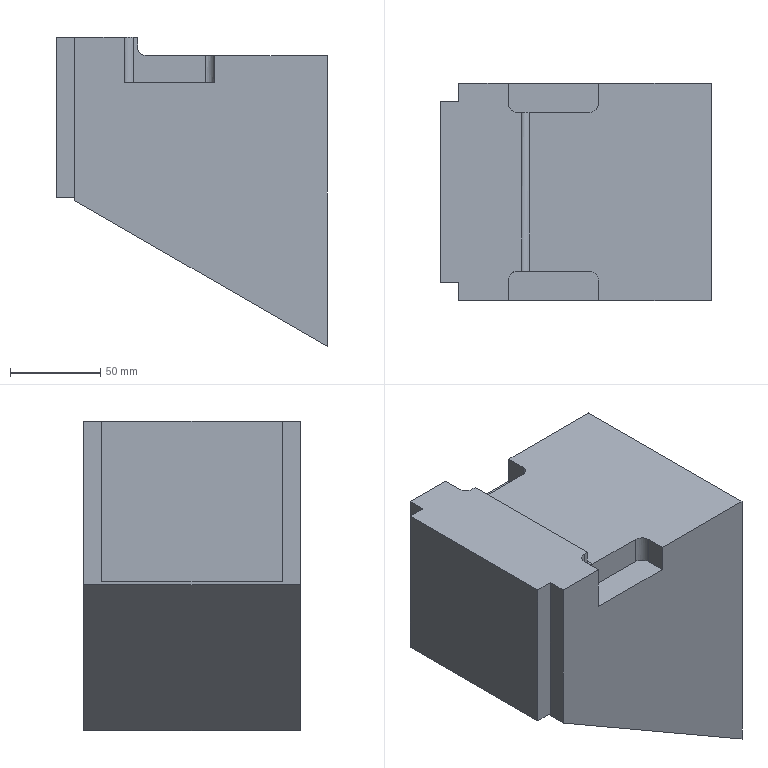Part | NX | features solid 2 | 1 solid | 25 faces | box 150 x 120 x 171.127 mm | volume 2133147 mm3 | plane 20 | cylinder 5 | commonest cylinder face diameters 10 x4 8 x1
STEP:
#1=CARTESIAN_POINT('',(-940.5,68.,-30.));
#2=VERTEX_POINT('',#1);
#3=CARTESIAN_POINT('',(-940.5,68.,-55.));
#4=VERTEX_POINT('',#3);
#5=CARTESIAN_POINT('',(-940.5,68.,-30.));
#6=CARTESIAN_POINT('',(-940.5,68.,-38.333));
#7=CARTESIAN_POINT('',(-940.5,68.,-46.667));
#8=CARTESIAN_POINT('',(-940.5,68.,-55.));
#9=B_SPLINE_CURVE_WITH_KNOTS('',3,(#5,#6,#7,#8),.UNSPECIFIED.,.F.,.F.,(4,4),(0.,1.),.UNSPECIFIED.);
#10=EDGE_CURVE('',#2,#4,#9,.T.);
#11=ORIENTED_EDGE('',*,*,#10,.T.);
#12=CARTESIAN_POINT('',(-890.5,68.,-55.));
#13=VERTEX_POINT('',#12);
#14=CARTESIAN_POINT('',(-940.5,68.,-55.));
#15=CARTESIAN_POINT('',(-923.833,68.,-55.));
#16=CARTESIAN_POINT('',(-907.167,68.,-55.));
#17=CARTESIAN_POINT('',(-890.5,68.,-55.));
#18=B_SPLINE_CURVE_WITH_KNOTS('',3,(#14,#15,#16,#17),.UNSPECIFIED.,.F.,.F.,(4,4),(0.,1.),.UNSPECIFIED.);
#19=EDGE_CURVE('',#4,#13,#18,.T.);
#20=ORIENTED_EDGE('',*,*,#19,.T.);
#21=CARTESIAN_POINT('',(-890.5,68.,-40.));
#22=VERTEX_POINT('',#21);
#23=CARTESIAN_POINT('',(-890.5,68.,-55.));
#24=CARTESIAN_POINT('',(-890.5,68.,-50.));
#25=CARTESIAN_POINT('',(-890.5,68.,-45.));
#26=CARTESIAN_POINT('',(-890.5,68.,-40.));
#27=B_SPLINE_CURVE_WITH_KNOTS('',3,(#23,#24,#25,#26),.UNSPECIFIED.,.F.,.F.,(4,4),(0.,1.),.UNSPECIFIED.);
#28=EDGE_CURVE('',#13,#22,#27,.T.);
#29=ORIENTED_EDGE('',*,*,#28,.T.);
#30=CARTESIAN_POINT('',(-828.,68.,-40.));
#31=VERTEX_POINT('',#30);
#32=CARTESIAN_POINT('',(-890.5,68.,-40.));
#33=CARTESIAN_POINT('',(-869.667,68.,-40.));
#34=CARTESIAN_POINT('',(-848.833,68.,-40.));
#35=CARTESIAN_POINT('',(-828.,68.,-40.));
#36=B_SPLINE_CURVE_WITH_KNOTS('',3,(#32,#33,#34,#35),.UNSPECIFIED.,.F.,.F.,(4,4),(0.,1.),.UNSPECIFIED.);
#37=EDGE_CURVE('',#22,#31,#36,.T.);
#38=ORIENTED_EDGE('',*,*,#37,.T.);
#39=CARTESIAN_POINT('',(-828.,68.,-201.127));
#40=VERTEX_POINT('',#39);
#41=CARTESIAN_POINT('',(-828.,68.,-40.));
#42=CARTESIAN_POINT('',(-828.,68.,-93.709));
#43=CARTESIAN_POINT('',(-828.,68.,-147.418));
#44=CARTESIAN_POINT('',(-828.,68.,-201.127));
#45=B_SPLINE_CURVE_WITH_KNOTS('',3,(#41,#42,#43,#44),.UNSPECIFIED.,.F.,.F.,(4,4),(0.,1.),.UNSPECIFIED.);
#46=EDGE_CURVE('',#31,#40,#45,.T.);
#47=ORIENTED_EDGE('',*,*,#46,.T.);
#48=CARTESIAN_POINT('',(-968.,68.,-120.298));
#49=VERTEX_POINT('',#48);
#50=CARTESIAN_POINT('',(-828.,68.,-201.127));
#51=CARTESIAN_POINT('',(-874.667,68.,-174.184));
#52=CARTESIAN_POINT('',(-921.333,68.,-147.241));
#53=CARTESIAN_POINT('',(-968.,68.,-120.298));
#54=B_SPLINE_CURVE_WITH_KNOTS('',3,(#50,#51,#52,#53),.UNSPECIFIED.,.F.,.F.,(4,4),(0.,1.),.UNSPECIFIED.);
#55=EDGE_CURVE('',#40,#49,#54,.T.);
#56=ORIENTED_EDGE('',*,*,#55,.T.);
#57=CARTESIAN_POINT('',(-968.,68.,-30.));
#58=VERTEX_POINT('',#57);
#59=CARTESIAN_POINT('',(-968.,68.,-120.298));
#60=CARTESIAN_POINT('',(-968.,68.,-90.199));
#61=CARTESIAN_POINT('',(-968.,68.,-60.099));
#62=CARTESIAN_POINT('',(-968.,68.,-30.));
#63=B_SPLINE_CURVE_WITH_KNOTS('',3,(#59,#60,#61,#62),.UNSPECIFIED.,.F.,.F.,(4,4),(0.,1.),.UNSPECIFIED.);
#64=EDGE_CURVE('',#49,#58,#63,.T.);
#65=ORIENTED_EDGE('',*,*,#64,.T.);
#66=CARTESIAN_POINT('',(-968.,68.,-30.));
#67=CARTESIAN_POINT('',(-958.833,68.,-30.));
#68=CARTESIAN_POINT('',(-949.667,68.,-30.));
#69=CARTESIAN_POINT('',(-940.5,68.,-30.));
#70=B_SPLINE_CURVE_WITH_KNOTS('',3,(#66,#67,#68,#69),.UNSPECIFIED.,.F.,.F.,(4,4),(0.,1.),.UNSPECIFIED.);
#71=EDGE_CURVE('',#58,#2,#70,.T.);
#72=ORIENTED_EDGE('',*,*,#71,.T.);
#73=EDGE_LOOP('',(#11,#20,#29,#38,#47,#56,#65,#72));
#74=FACE_BOUND('',#73,.T.);
#75=CARTESIAN_POINT('',(-898.,68.,-115.564));
#76=DIRECTION('',(0.,1.,0.));
#77=DIRECTION('',(-1.,0.,0.));
#78=AXIS2_PLACEMENT_3D('',#75,#76,#77);
#79=PLANE('',#78);
#80=ADVANCED_FACE('',(#74),#79,.T.);
#81=ORIENTED_EDGE('',*,*,#19,.F.);
#82=CARTESIAN_POINT('',(-940.5,57.,-55.));
#83=VERTEX_POINT('',#82);
#84=CARTESIAN_POINT('',(-940.5,68.,-55.));
#85=CARTESIAN_POINT('',(-940.5,64.333,-55.));
#86=CARTESIAN_POINT('',(-940.5,60.667,-55.));
#87=CARTESIAN_POINT('',(-940.5,57.,-55.));
#88=B_SPLINE_CURVE_WITH_KNOTS('',3,(#84,#85,#86,#87),.UNSPECIFIED.,.F.,.F.,(4,4),(0.,1.),.UNSPECIFIED.);
#89=EDGE_CURVE('',#4,#83,#88,.T.);
#90=ORIENTED_EDGE('',*,*,#89,.T.);
#91=CARTESIAN_POINT('',(-935.5,52.,-55.));
#92=VERTEX_POINT('',#91);
#93=CARTESIAN_POINT('',(-940.5,57.,-55.));
#94=CARTESIAN_POINT('',(-940.499,56.892,-55.));
#95=CARTESIAN_POINT('',(-940.497,56.767,-55.));
#96=CARTESIAN_POINT('',(-940.472,56.422,-55.));
#97=CARTESIAN_POINT('',(-940.388,55.867,-55.));
#98=CARTESIAN_POINT('',(-940.15,55.074,-55.));
#99=CARTESIAN_POINT('',(-939.686,54.208,-55.));
#100=CARTESIAN_POINT('',(-939.059,53.441,-55.));
#101=CARTESIAN_POINT('',(-938.293,52.815,-55.));
#102=CARTESIAN_POINT('',(-937.426,52.35,-55.));
#103=CARTESIAN_POINT('',(-936.633,52.113,-55.));
#104=CARTESIAN_POINT('',(-936.079,52.026,-55.));
#105=CARTESIAN_POINT('',(-935.733,52.006,-55.));
#106=CARTESIAN_POINT('',(-935.609,52.003,-55.));
#107=CARTESIAN_POINT('',(-935.5,52.,-55.));
#108=B_SPLINE_CURVE_WITH_KNOTS('',3,(#93,#94,#95,#96,#97,#98,#99,#100,#101,#102,#103,#104,#105,#106,#107),.UNSPECIFIED.,.F.,.F.,(4,1,1,1,1,1,1,1,1,1,1,1,4),(0.,0.03125,0.0625,0.125,0.25,0.375,0.5,0.625,0.75,0.875,0.9375,0.9688,1.),.UNSPECIFIED.);
#109=EDGE_CURVE('',#83,#92,#108,.T.);
#110=ORIENTED_EDGE('',*,*,#109,.T.);
#111=CARTESIAN_POINT('',(-895.5,52.,-55.));
#112=VERTEX_POINT('',#111);
#113=CARTESIAN_POINT('',(-935.5,52.,-55.));
#114=CARTESIAN_POINT('',(-922.167,52.,-55.));
#115=CARTESIAN_POINT('',(-908.833,52.,-55.));
#116=CARTESIAN_POINT('',(-895.5,52.,-55.));
#117=B_SPLINE_CURVE_WITH_KNOTS('',3,(#113,#114,#115,#116),.UNSPECIFIED.,.F.,.F.,(4,4),(0.,1.),.UNSPECIFIED.);
#118=EDGE_CURVE('',#92,#112,#117,.T.);
#119=ORIENTED_EDGE('',*,*,#118,.T.);
#120=CARTESIAN_POINT('',(-890.5,57.,-55.));
#121=VERTEX_POINT('',#120);
#122=CARTESIAN_POINT('',(-895.5,52.,-55.));
#123=CARTESIAN_POINT('',(-895.392,52.001,-55.));
#124=CARTESIAN_POINT('',(-895.267,52.003,-55.));
#125=CARTESIAN_POINT('',(-894.922,52.028,-55.));
#126=CARTESIAN_POINT('',(-894.367,52.112,-55.));
#127=CARTESIAN_POINT('',(-893.574,52.35,-55.));
#128=CARTESIAN_POINT('',(-892.708,52.814,-55.));
#129=CARTESIAN_POINT('',(-891.941,53.441,-55.));
#130=CARTESIAN_POINT('',(-891.315,54.207,-55.));
#131=CARTESIAN_POINT('',(-890.85,55.074,-55.));
#132=CARTESIAN_POINT('',(-890.613,55.867,-55.));
#133=CARTESIAN_POINT('',(-890.526,56.421,-55.));
#134=CARTESIAN_POINT('',(-890.506,56.767,-55.));
#135=CARTESIAN_POINT('',(-890.503,56.891,-55.));
#136=CARTESIAN_POINT('',(-890.5,57.,-55.));
#137=B_SPLINE_CURVE_WITH_KNOTS('',3,(#122,#123,#124,#125,#126,#127,#128,#129,#130,#131,#132,#133,#134,#135,#136),.UNSPECIFIED.,.F.,.F.,(4,1,1,1,1,1,1,1,1,1,1,1,4),(0.,0.03125,0.0625,0.125,0.25,0.375,0.5,0.625,0.75,0.875,0.9375,0.9688,1.),.UNSPECIFIED.);
#138=EDGE_CURVE('',#112,#121,#137,.T.);
#139=ORIENTED_EDGE('',*,*,#138,.T.);
#140=CARTESIAN_POINT('',(-890.5,57.,-55.));
#141=CARTESIAN_POINT('',(-890.5,60.667,-55.));
#142=CARTESIAN_POINT('',(-890.5,64.333,-55.));
#143=CARTESIAN_POINT('',(-890.5,68.,-55.));
#144=B_SPLINE_CURVE_WITH_KNOTS('',3,(#140,#141,#142,#143),.UNSPECIFIED.,.F.,.F.,(4,4),(0.,1.),.UNSPECIFIED.);
#145=EDGE_CURVE('',#121,#13,#144,.T.);
#146=ORIENTED_EDGE('',*,*,#145,.T.);
#147=EDGE_LOOP('',(#81,#90,#110,#119,#139,#146));
#148=FACE_BOUND('',#147,.T.);
#149=CARTESIAN_POINT('',(-915.5,60.,-55.));
#150=DIRECTION('',(0.,0.,1.));
#151=DIRECTION('',(0.,-1.,0.));
#152=AXIS2_PLACEMENT_3D('',#149,#150,#151);
#153=PLANE('',#152);
#154=ADVANCED_FACE('',(#148),#153,.T.);
#155=CARTESIAN_POINT('',(-940.5,57.,-30.));
#156=VERTEX_POINT('',#155);
#157=CARTESIAN_POINT('',(-940.5,68.,-30.));
#158=CARTESIAN_POINT('',(-940.5,64.333,-30.));
#159=CARTESIAN_POINT('',(-940.5,60.667,-30.));
#160=CARTESIAN_POINT('',(-940.5,57.,-30.));
#161=B_SPLINE_CURVE_WITH_KNOTS('',3,(#157,#158,#159,#160),.UNSPECIFIED.,.F.,.F.,(4,4),(0.,1.),.UNSPECIFIED.);
#162=EDGE_CURVE('',#2,#156,#161,.T.);
#163=ORIENTED_EDGE('',*,*,#162,.T.);
#164=CARTESIAN_POINT('',(-940.5,57.,-30.));
#165=CARTESIAN_POINT('',(-940.5,57.,-38.333));
#166=CARTESIAN_POINT('',(-940.5,57.,-46.667));
#167=CARTESIAN_POINT('',(-940.5,57.,-55.));
#168=B_SPLINE_CURVE_WITH_KNOTS('',3,(#164,#165,#166,#167),.UNSPECIFIED.,.F.,.F.,(4,4),(0.,1.),.UNSPECIFIED.);
#169=EDGE_CURVE('',#156,#83,#168,.T.);
#170=ORIENTED_EDGE('',*,*,#169,.T.);
#171=ORIENTED_EDGE('',*,*,#89,.F.);
#172=ORIENTED_EDGE('',*,*,#10,.F.);
#173=EDGE_LOOP('',(#163,#170,#171,#172));
#174=FACE_BOUND('',#173,.T.);
#175=CARTESIAN_POINT('',(-940.5,62.5,-42.5));
#176=DIRECTION('',(1.,0.,0.));
#177=DIRECTION('',(0.,1.,0.));
#178=AXIS2_PLACEMENT_3D('',#175,#176,#177);
#179=PLANE('',#178);
#180=ADVANCED_FACE('',(#174),#179,.T.);
#181=CARTESIAN_POINT('',(-935.5,-36.,-30.));
#182=VERTEX_POINT('',#181);
#183=CARTESIAN_POINT('',(-933.,-36.,-30.));
#184=VERTEX_POINT('',#183);
#185=CARTESIAN_POINT('',(-935.5,-36.,-30.));
#186=CARTESIAN_POINT('',(-934.667,-36.,-30.));
#187=CARTESIAN_POINT('',(-933.833,-36.,-30.));
#188=CARTESIAN_POINT('',(-933.,-36.,-30.));
#189=B_SPLINE_CURVE_WITH_KNOTS('',3,(#185,#186,#187,#188),.UNSPECIFIED.,.F.,.F.,(4,4),(0.,1.),.UNSPECIFIED.);
#190=EDGE_CURVE('',#182,#184,#189,.T.);
#191=ORIENTED_EDGE('',*,*,#190,.T.);
#192=CARTESIAN_POINT('',(-933.,52.,-30.));
#193=VERTEX_POINT('',#192);
#194=CARTESIAN_POINT('',(-933.,-36.,-30.));
#195=CARTESIAN_POINT('',(-933.,-6.667,-30.));
#196=CARTESIAN_POINT('',(-933.,22.667,-30.));
#197=CARTESIAN_POINT('',(-933.,52.,-30.));
#198=B_SPLINE_CURVE_WITH_KNOTS('',3,(#194,#195,#196,#197),.UNSPECIFIED.,.F.,.F.,(4,4),(0.,1.),.UNSPECIFIED.);
#199=EDGE_CURVE('',#184,#193,#198,.T.);
#200=ORIENTED_EDGE('',*,*,#199,.T.);
#201=CARTESIAN_POINT('',(-935.5,52.,-30.));
#202=VERTEX_POINT('',#201);
#203=CARTESIAN_POINT('',(-933.,52.,-30.));
#204=CARTESIAN_POINT('',(-933.833,52.,-30.));
#205=CARTESIAN_POINT('',(-934.667,52.,-30.));
#206=CARTESIAN_POINT('',(-935.5,52.,-30.));
#207=B_SPLINE_CURVE_WITH_KNOTS('',3,(#203,#204,#205,#206),.UNSPECIFIED.,.F.,.F.,(4,4),(0.,1.),.UNSPECIFIED.);
#208=EDGE_CURVE('',#193,#202,#207,.T.);
#209=ORIENTED_EDGE('',*,*,#208,.T.);
#210=CARTESIAN_POINT('',(-935.5,52.,-30.));
#211=CARTESIAN_POINT('',(-935.608,52.001,-30.));
#212=CARTESIAN_POINT('',(-935.733,52.003,-30.));
#213=CARTESIAN_POINT('',(-936.078,52.028,-30.));
#214=CARTESIAN_POINT('',(-936.633,52.112,-30.));
#215=CARTESIAN_POINT('',(-937.426,52.35,-30.));
#216=CARTESIAN_POINT('',(-938.292,52.814,-30.));
#217=CARTESIAN_POINT('',(-939.059,53.441,-30.));
#218=CARTESIAN_POINT('',(-939.685,54.207,-30.));
#219=CARTESIAN_POINT('',(-940.15,55.074,-30.));
#220=CARTESIAN_POINT('',(-940.387,55.867,-30.));
#221=CARTESIAN_POINT('',(-940.474,56.421,-30.));
#222=CARTESIAN_POINT('',(-940.494,56.767,-30.));
#223=CARTESIAN_POINT('',(-940.497,56.891,-30.));
#224=CARTESIAN_POINT('',(-940.5,57.,-30.));
#225=B_SPLINE_CURVE_WITH_KNOTS('',3,(#210,#211,#212,#213,#214,#215,#216,#217,#218,#219,#220,#221,#222,#223,#224),.UNSPECIFIED.,.F.,.F.,(4,1,1,1,1,1,1,1,1,1,1,1,4),(0.,0.03125,0.0625,0.125,0.25,0.375,0.5,0.625,0.75,0.875,0.9375,0.9688,1.),.UNSPECIFIED.);
#226=EDGE_CURVE('',#202,#156,#225,.T.);
#227=ORIENTED_EDGE('',*,*,#226,.T.);
#228=ORIENTED_EDGE('',*,*,#162,.F.);
#229=ORIENTED_EDGE('',*,*,#71,.F.);
#230=CARTESIAN_POINT('',(-968.,58.,-30.));
#231=VERTEX_POINT('',#230);
#232=CARTESIAN_POINT('',(-968.,68.,-30.));
#233=CARTESIAN_POINT('',(-968.,64.667,-30.));
#234=CARTESIAN_POINT('',(-968.,61.333,-30.));
#235=CARTESIAN_POINT('',(-968.,58.,-30.));
#236=B_SPLINE_CURVE_WITH_KNOTS('',3,(#232,#233,#234,#235),.UNSPECIFIED.,.F.,.F.,(4,4),(0.,1.),.UNSPECIFIED.);
#237=EDGE_CURVE('',#58,#231,#236,.T.);
#238=ORIENTED_EDGE('',*,*,#237,.T.);
#239=CARTESIAN_POINT('',(-978.,58.,-30.));
#240=VERTEX_POINT('',#239);
#241=CARTESIAN_POINT('',(-968.,58.,-30.));
#242=CARTESIAN_POINT('',(-971.333,58.,-30.));
#243=CARTESIAN_POINT('',(-974.667,58.,-30.));
#244=CARTESIAN_POINT('',(-978.,58.,-30.));
#245=B_SPLINE_CURVE_WITH_KNOTS('',3,(#241,#242,#243,#244),.UNSPECIFIED.,.F.,.F.,(4,4),(0.,1.),.UNSPECIFIED.);
#246=EDGE_CURVE('',#231,#240,#245,.T.);
#247=ORIENTED_EDGE('',*,*,#246,.T.);
#248=CARTESIAN_POINT('',(-978.,-42.,-30.));
#249=VERTEX_POINT('',#248);
#250=CARTESIAN_POINT('',(-978.,58.,-30.));
#251=CARTESIAN_POINT('',(-978.,24.667,-30.));
#252=CARTESIAN_POINT('',(-978.,-8.667,-30.));
#253=CARTESIAN_POINT('',(-978.,-42.,-30.));
#254=B_SPLINE_CURVE_WITH_KNOTS('',3,(#250,#251,#252,#253),.UNSPECIFIED.,.F.,.F.,(4,4),(0.,1.),.UNSPECIFIED.);
#255=EDGE_CURVE('',#240,#249,#254,.T.);
#256=ORIENTED_EDGE('',*,*,#255,.T.);
#257=CARTESIAN_POINT('',(-968.,-42.,-30.));
#258=VERTEX_POINT('',#257);
#259=CARTESIAN_POINT('',(-978.,-42.,-30.));
#260=CARTESIAN_POINT('',(-974.667,-42.,-30.));
#261=CARTESIAN_POINT('',(-971.333,-42.,-30.));
#262=CARTESIAN_POINT('',(-968.,-42.,-30.));
#263=B_SPLINE_CURVE_WITH_KNOTS('',3,(#259,#260,#261,#262),.UNSPECIFIED.,.F.,.F.,(4,4),(0.,1.),.UNSPECIFIED.);
#264=EDGE_CURVE('',#249,#258,#263,.T.);
#265=ORIENTED_EDGE('',*,*,#264,.T.);
#266=CARTESIAN_POINT('',(-968.,-52.,-30.));
#267=VERTEX_POINT('',#266);
#268=CARTESIAN_POINT('',(-968.,-42.,-30.));
#269=CARTESIAN_POINT('',(-968.,-45.333,-30.));
#270=CARTESIAN_POINT('',(-968.,-48.667,-30.));
#271=CARTESIAN_POINT('',(-968.,-52.,-30.));
#272=B_SPLINE_CURVE_WITH_KNOTS('',3,(#268,#269,#270,#271),.UNSPECIFIED.,.F.,.F.,(4,4),(0.,1.),.UNSPECIFIED.);
#273=EDGE_CURVE('',#258,#267,#272,.T.);
#274=ORIENTED_EDGE('',*,*,#273,.T.);
#275=CARTESIAN_POINT('',(-940.5,-52.,-30.));
#276=VERTEX_POINT('',#275);
#277=CARTESIAN_POINT('',(-968.,-52.,-30.));
#278=CARTESIAN_POINT('',(-958.833,-52.,-30.));
#279=CARTESIAN_POINT('',(-949.667,-52.,-30.));
#280=CARTESIAN_POINT('',(-940.5,-52.,-30.));
#281=B_SPLINE_CURVE_WITH_KNOTS('',3,(#277,#278,#279,#280),.UNSPECIFIED.,.F.,.F.,(4,4),(0.,1.),.UNSPECIFIED.);
#282=EDGE_CURVE('',#267,#276,#281,.T.);
#283=ORIENTED_EDGE('',*,*,#282,.T.);
#284=CARTESIAN_POINT('',(-940.5,-41.,-30.));
#285=VERTEX_POINT('',#284);
#286=CARTESIAN_POINT('',(-940.5,-52.,-30.));
#287=CARTESIAN_POINT('',(-940.5,-48.333,-30.));
#288=CARTESIAN_POINT('',(-940.5,-44.667,-30.));
#289=CARTESIAN_POINT('',(-940.5,-41.,-30.));
#290=B_SPLINE_CURVE_WITH_KNOTS('',3,(#286,#287,#288,#289),.UNSPECIFIED.,.F.,.F.,(4,4),(0.,1.),.UNSPECIFIED.);
#291=EDGE_CURVE('',#276,#285,#290,.T.);
#292=ORIENTED_EDGE('',*,*,#291,.T.);
#293=CARTESIAN_POINT('',(-940.5,-41.,-30.));
#294=CARTESIAN_POINT('',(-940.499,-40.892,-30.));
#295=CARTESIAN_POINT('',(-940.497,-40.767,-30.));
#296=CARTESIAN_POINT('',(-940.472,-40.422,-30.));
#297=CARTESIAN_POINT('',(-940.388,-39.867,-30.));
#298=CARTESIAN_POINT('',(-940.15,-39.074,-30.));
#299=CARTESIAN_POINT('',(-939.686,-38.208,-30.));
#300=CARTESIAN_POINT('',(-939.059,-37.441,-30.));
#301=CARTESIAN_POINT('',(-938.293,-36.815,-30.));
#302=CARTESIAN_POINT('',(-937.426,-36.35,-30.));
#303=CARTESIAN_POINT('',(-936.633,-36.113,-30.));
#304=CARTESIAN_POINT('',(-936.079,-36.026,-30.));
#305=CARTESIAN_POINT('',(-935.733,-36.006,-30.));
#306=CARTESIAN_POINT('',(-935.609,-36.003,-30.));
#307=CARTESIAN_POINT('',(-935.5,-36.,-30.));
#308=B_SPLINE_CURVE_WITH_KNOTS('',3,(#293,#294,#295,#296,#297,#298,#299,#300,#301,#302,#303,#304,#305,#306,#307),.UNSPECIFIED.,.F.,.F.,(4,1,1,1,1,1,1,1,1,1,1,1,4),(0.,0.03125,0.0625,0.125,0.25,0.375,0.5,0.625,0.75,0.875,0.9375,0.9688,1.),.UNSPECIFIED.);
#309=EDGE_CURVE('',#285,#182,#308,.T.);
#310=ORIENTED_EDGE('',*,*,#309,.T.);
#311=EDGE_LOOP('',(#191,#200,#209,#227,#228,#229,#238,#247,#256,#265,#274,#283,#292,#310));
#312=FACE_BOUND('',#311,.T.);
#313=CARTESIAN_POINT('',(-955.5,8.,-30.));
#314=DIRECTION('',(0.,0.,1.));
#315=DIRECTION('',(0.,-1.,0.));
#316=AXIS2_PLACEMENT_3D('',#313,#314,#315);
#317=PLANE('',#316);
#318=ADVANCED_FACE('',(#312),#317,.T.);
#319=CARTESIAN_POINT('',(-968.,-42.,-118.845));
#320=VERTEX_POINT('',#319);
#321=CARTESIAN_POINT('',(-968.,-42.,-30.));
#322=CARTESIAN_POINT('',(-968.,-42.,-59.615));
#323=CARTESIAN_POINT('',(-968.,-42.,-89.23));
#324=CARTESIAN_POINT('',(-968.,-42.,-118.845));
#325=B_SPLINE_CURVE_WITH_KNOTS('',3,(#321,#322,#323,#324),.UNSPECIFIED.,.F.,.F.,(4,4),(0.,1.),.UNSPECIFIED.);
#326=EDGE_CURVE('',#258,#320,#325,.T.);
#327=ORIENTED_EDGE('',*,*,#326,.T.);
#328=CARTESIAN_POINT('',(-968.,58.,-118.845));
#329=VERTEX_POINT('',#328);
#330=CARTESIAN_POINT('',(-968.,-42.,-118.845));
#331=CARTESIAN_POINT('',(-968.,-8.667,-118.845));
#332=CARTESIAN_POINT('',(-968.,24.667,-118.845));
#333=CARTESIAN_POINT('',(-968.,58.,-118.845));
#334=B_SPLINE_CURVE_WITH_KNOTS('',3,(#330,#331,#332,#333),.UNSPECIFIED.,.F.,.F.,(4,4),(0.,1.),.UNSPECIFIED.);
#335=EDGE_CURVE('',#320,#329,#334,.T.);
#336=ORIENTED_EDGE('',*,*,#335,.T.);
#337=CARTESIAN_POINT('',(-968.,58.,-118.845));
#338=CARTESIAN_POINT('',(-968.,58.,-89.23));
#339=CARTESIAN_POINT('',(-968.,58.,-59.615));
#340=CARTESIAN_POINT('',(-968.,58.,-30.));
#341=B_SPLINE_CURVE_WITH_KNOTS('',3,(#337,#338,#339,#340),.UNSPECIFIED.,.F.,.F.,(4,4),(0.,1.),.UNSPECIFIED.);
#342=EDGE_CURVE('',#329,#231,#341,.T.);
#343=ORIENTED_EDGE('',*,*,#342,.T.);
#344=ORIENTED_EDGE('',*,*,#237,.F.);
#345=ORIENTED_EDGE('',*,*,#64,.F.);
#346=CARTESIAN_POINT('',(-968.,-52.,-120.298));
#347=VERTEX_POINT('',#346);
#348=CARTESIAN_POINT('',(-968.,68.,-120.298));
#349=CARTESIAN_POINT('',(-968.,28.,-120.298));
#350=CARTESIAN_POINT('',(-968.,-12.,-120.298));
#351=CARTESIAN_POINT('',(-968.,-52.,-120.298));
#352=B_SPLINE_CURVE_WITH_KNOTS('',3,(#348,#349,#350,#351),.UNSPECIFIED.,.F.,.F.,(4,4),(0.,1.),.UNSPECIFIED.);
#353=EDGE_CURVE('',#49,#347,#352,.T.);
#354=ORIENTED_EDGE('',*,*,#353,.T.);
#355=CARTESIAN_POINT('',(-968.,-52.,-120.298));
#356=CARTESIAN_POINT('',(-968.,-52.,-90.199));
#357=CARTESIAN_POINT('',(-968.,-52.,-60.099));
#358=CARTESIAN_POINT('',(-968.,-52.,-30.));
#359=B_SPLINE_CURVE_WITH_KNOTS('',3,(#355,#356,#357,#358),.UNSPECIFIED.,.F.,.F.,(4,4),(0.,1.),.UNSPECIFIED.);
#360=EDGE_CURVE('',#347,#267,#359,.T.);
#361=ORIENTED_EDGE('',*,*,#360,.T.);
#362=ORIENTED_EDGE('',*,*,#273,.F.);
#363=EDGE_LOOP('',(#327,#336,#343,#344,#345,#354,#361,#362));
#364=FACE_BOUND('',#363,.T.);
#365=CARTESIAN_POINT('',(-968.,8.,-75.149));
#366=DIRECTION('',(-1.,0.,0.));
#367=DIRECTION('',(0.,-1.,0.));
#368=AXIS2_PLACEMENT_3D('',#365,#366,#367);
#369=PLANE('',#368);
#370=ADVANCED_FACE('',(#364),#369,.T.);
#371=ORIENTED_EDGE('',*,*,#55,.F.);
#372=CARTESIAN_POINT('',(-828.,-52.,-201.127));
#373=VERTEX_POINT('',#372);
#374=CARTESIAN_POINT('',(-828.,68.,-201.127));
#375=CARTESIAN_POINT('',(-828.,28.,-201.127));
#376=CARTESIAN_POINT('',(-828.,-12.,-201.127));
#377=CARTESIAN_POINT('',(-828.,-52.,-201.127));
#378=B_SPLINE_CURVE_WITH_KNOTS('',3,(#374,#375,#376,#377),.UNSPECIFIED.,.F.,.F.,(4,4),(0.,1.),.UNSPECIFIED.);
#379=EDGE_CURVE('',#40,#373,#378,.T.);
#380=ORIENTED_EDGE('',*,*,#379,.T.);
#381=CARTESIAN_POINT('',(-828.,-52.,-201.127));
#382=CARTESIAN_POINT('',(-874.667,-52.,-174.184));
#383=CARTESIAN_POINT('',(-921.333,-52.,-147.241));
#384=CARTESIAN_POINT('',(-968.,-52.,-120.298));
#385=B_SPLINE_CURVE_WITH_KNOTS('',3,(#381,#382,#383,#384),.UNSPECIFIED.,.F.,.F.,(4,4),(0.,1.),.UNSPECIFIED.);
#386=EDGE_CURVE('',#373,#347,#385,.T.);
#387=ORIENTED_EDGE('',*,*,#386,.T.);
#388=ORIENTED_EDGE('',*,*,#353,.F.);
#389=EDGE_LOOP('',(#371,#380,#387,#388));
#390=FACE_BOUND('',#389,.T.);
#391=CARTESIAN_POINT('',(-898.,8.,-160.713));
#392=DIRECTION('',(-0.5,0.,-0.866));
#393=DIRECTION('',(0.866,0.,-0.5));
#394=AXIS2_PLACEMENT_3D('',#391,#392,#393);
#395=PLANE('',#394);
#396=ADVANCED_FACE('',(#390),#395,.T.);
#397=ORIENTED_EDGE('',*,*,#46,.F.);
#398=CARTESIAN_POINT('',(-828.,-52.,-40.));
#399=VERTEX_POINT('',#398);
#400=CARTESIAN_POINT('',(-828.,68.,-40.));
#401=CARTESIAN_POINT('',(-828.,28.,-40.));
#402=CARTESIAN_POINT('',(-828.,-12.,-40.));
#403=CARTESIAN_POINT('',(-828.,-52.,-40.));
#404=B_SPLINE_CURVE_WITH_KNOTS('',3,(#400,#401,#402,#403),.UNSPECIFIED.,.F.,.F.,(4,4),(0.,1.),.UNSPECIFIED.);
#405=EDGE_CURVE('',#31,#399,#404,.T.);
#406=ORIENTED_EDGE('',*,*,#405,.T.);
#407=CARTESIAN_POINT('',(-828.,-52.,-40.));
#408=CARTESIAN_POINT('',(-828.,-52.,-93.709));
#409=CARTESIAN_POINT('',(-828.,-52.,-147.418));
#410=CARTESIAN_POINT('',(-828.,-52.,-201.127));
#411=B_SPLINE_CURVE_WITH_KNOTS('',3,(#407,#408,#409,#410),.UNSPECIFIED.,.F.,.F.,(4,4),(0.,1.),.UNSPECIFIED.);
#412=EDGE_CURVE('',#399,#373,#411,.T.);
#413=ORIENTED_EDGE('',*,*,#412,.T.);
#414=ORIENTED_EDGE('',*,*,#379,.F.);
#415=EDGE_LOOP('',(#397,#406,#413,#414));
#416=FACE_BOUND('',#415,.T.);
#417=CARTESIAN_POINT('',(-828.,8.,-120.564));
#418=DIRECTION('',(1.,0.,0.));
#419=DIRECTION('',(0.,1.,0.));
#420=AXIS2_PLACEMENT_3D('',#417,#418,#419);
#421=PLANE('',#420);
#422=ADVANCED_FACE('',(#416),#421,.T.);
#423=CARTESIAN_POINT('',(-890.5,57.,-40.));
#424=VERTEX_POINT('',#423);
#425=CARTESIAN_POINT('',(-890.5,68.,-40.));
#426=CARTESIAN_POINT('',(-890.5,64.333,-40.));
#427=CARTESIAN_POINT('',(-890.5,60.667,-40.));
#428=CARTESIAN_POINT('',(-890.5,57.,-40.));
#429=B_SPLINE_CURVE_WITH_KNOTS('',3,(#425,#426,#427,#428),.UNSPECIFIED.,.F.,.F.,(4,4),(0.,1.),.UNSPECIFIED.);
#430=EDGE_CURVE('',#22,#424,#429,.T.);
#431=ORIENTED_EDGE('',*,*,#430,.T.);
#432=CARTESIAN_POINT('',(-895.5,52.,-40.));
#433=VERTEX_POINT('',#432);
#434=CARTESIAN_POINT('',(-890.5,57.,-40.));
#435=CARTESIAN_POINT('',(-890.501,56.892,-40.));
#436=CARTESIAN_POINT('',(-890.503,56.767,-40.));
#437=CARTESIAN_POINT('',(-890.528,56.422,-40.));
#438=CARTESIAN_POINT('',(-890.612,55.867,-40.));
#439=CARTESIAN_POINT('',(-890.85,55.074,-40.));
#440=CARTESIAN_POINT('',(-891.314,54.208,-40.));
#441=CARTESIAN_POINT('',(-891.941,53.441,-40.));
#442=CARTESIAN_POINT('',(-892.707,52.815,-40.));
#443=CARTESIAN_POINT('',(-893.574,52.35,-40.));
#444=CARTESIAN_POINT('',(-894.367,52.113,-40.));
#445=CARTESIAN_POINT('',(-894.921,52.026,-40.));
#446=CARTESIAN_POINT('',(-895.267,52.006,-40.));
#447=CARTESIAN_POINT('',(-895.391,52.003,-40.));
#448=CARTESIAN_POINT('',(-895.5,52.,-40.));
#449=B_SPLINE_CURVE_WITH_KNOTS('',3,(#434,#435,#436,#437,#438,#439,#440,#441,#442,#443,#444,#445,#446,#447,#448),.UNSPECIFIED.,.F.,.F.,(4,1,1,1,1,1,1,1,1,1,1,1,4),(0.,0.03125,0.0625,0.125,0.25,0.375,0.5,0.625,0.75,0.875,0.9375,0.9688,1.),.UNSPECIFIED.);
#450=EDGE_CURVE('',#424,#433,#449,.T.);
#451=ORIENTED_EDGE('',*,*,#450,.T.);
#452=CARTESIAN_POINT('',(-929.,52.,-40.));
#453=VERTEX_POINT('',#452);
#454=CARTESIAN_POINT('',(-895.5,52.,-40.));
#455=CARTESIAN_POINT('',(-906.667,52.,-40.));
#456=CARTESIAN_POINT('',(-917.833,52.,-40.));
#457=CARTESIAN_POINT('',(-929.,52.,-40.));
#458=B_SPLINE_CURVE_WITH_KNOTS('',3,(#454,#455,#456,#457),.UNSPECIFIED.,.F.,.F.,(4,4),(0.,1.),.UNSPECIFIED.);
#459=EDGE_CURVE('',#433,#453,#458,.T.);
#460=ORIENTED_EDGE('',*,*,#459,.T.);
#461=CARTESIAN_POINT('',(-929.,-36.,-40.));
#462=VERTEX_POINT('',#461);
#463=CARTESIAN_POINT('',(-929.,52.,-40.));
#464=CARTESIAN_POINT('',(-929.,22.667,-40.));
#465=CARTESIAN_POINT('',(-929.,-6.667,-40.));
#466=CARTESIAN_POINT('',(-929.,-36.,-40.));
#467=B_SPLINE_CURVE_WITH_KNOTS('',3,(#463,#464,#465,#466),.UNSPECIFIED.,.F.,.F.,(4,4),(0.,1.),.UNSPECIFIED.);
#468=EDGE_CURVE('',#453,#462,#467,.T.);
#469=ORIENTED_EDGE('',*,*,#468,.T.);
#470=CARTESIAN_POINT('',(-895.5,-36.,-40.));
#471=VERTEX_POINT('',#470);
#472=CARTESIAN_POINT('',(-929.,-36.,-40.));
#473=CARTESIAN_POINT('',(-917.833,-36.,-40.));
#474=CARTESIAN_POINT('',(-906.667,-36.,-40.));
#475=CARTESIAN_POINT('',(-895.5,-36.,-40.));
#476=B_SPLINE_CURVE_WITH_KNOTS('',3,(#472,#473,#474,#475),.UNSPECIFIED.,.F.,.F.,(4,4),(0.,1.),.UNSPECIFIED.);
#477=EDGE_CURVE('',#462,#471,#476,.T.);
#478=ORIENTED_EDGE('',*,*,#477,.T.);
#479=CARTESIAN_POINT('',(-890.5,-41.,-40.));
#480=VERTEX_POINT('',#479);
#481=CARTESIAN_POINT('',(-895.5,-36.,-40.));
#482=CARTESIAN_POINT('',(-895.392,-36.001,-40.));
#483=CARTESIAN_POINT('',(-895.267,-36.003,-40.));
#484=CARTESIAN_POINT('',(-894.922,-36.028,-40.));
#485=CARTESIAN_POINT('',(-894.367,-36.112,-40.));
#486=CARTESIAN_POINT('',(-893.574,-36.35,-40.));
#487=CARTESIAN_POINT('',(-892.708,-36.814,-40.));
#488=CARTESIAN_POINT('',(-891.941,-37.441,-40.));
#489=CARTESIAN_POINT('',(-891.315,-38.207,-40.));
#490=CARTESIAN_POINT('',(-890.85,-39.074,-40.));
#491=CARTESIAN_POINT('',(-890.613,-39.867,-40.));
#492=CARTESIAN_POINT('',(-890.526,-40.421,-40.));
#493=CARTESIAN_POINT('',(-890.506,-40.767,-40.));
#494=CARTESIAN_POINT('',(-890.503,-40.891,-40.));
#495=CARTESIAN_POINT('',(-890.5,-41.,-40.));
#496=B_SPLINE_CURVE_WITH_KNOTS('',3,(#481,#482,#483,#484,#485,#486,#487,#488,#489,#490,#491,#492,#493,#494,#495),.UNSPECIFIED.,.F.,.F.,(4,1,1,1,1,1,1,1,1,1,1,1,4),(0.,0.03125,0.0625,0.125,0.25,0.375,0.5,0.625,0.75,0.875,0.9375,0.9688,1.),.UNSPECIFIED.);
#497=EDGE_CURVE('',#471,#480,#496,.T.);
#498=ORIENTED_EDGE('',*,*,#497,.T.);
#499=CARTESIAN_POINT('',(-890.5,-52.,-40.));
#500=VERTEX_POINT('',#499);
#501=CARTESIAN_POINT('',(-890.5,-41.,-40.));
#502=CARTESIAN_POINT('',(-890.5,-44.667,-40.));
#503=CARTESIAN_POINT('',(-890.5,-48.333,-40.));
#504=CARTESIAN_POINT('',(-890.5,-52.,-40.));
#505=B_SPLINE_CURVE_WITH_KNOTS('',3,(#501,#502,#503,#504),.UNSPECIFIED.,.F.,.F.,(4,4),(0.,1.),.UNSPECIFIED.);
#506=EDGE_CURVE('',#480,#500,#505,.T.);
#507=ORIENTED_EDGE('',*,*,#506,.T.);
#508=CARTESIAN_POINT('',(-890.5,-52.,-40.));
#509=CARTESIAN_POINT('',(-869.667,-52.,-40.));
#510=CARTESIAN_POINT('',(-848.833,-52.,-40.));
#511=CARTESIAN_POINT('',(-828.,-52.,-40.));
#512=B_SPLINE_CURVE_WITH_KNOTS('',3,(#508,#509,#510,#511),.UNSPECIFIED.,.F.,.F.,(4,4),(0.,1.),.UNSPECIFIED.);
#513=EDGE_CURVE('',#500,#399,#512,.T.);
#514=ORIENTED_EDGE('',*,*,#513,.T.);
#515=ORIENTED_EDGE('',*,*,#405,.F.);
#516=ORIENTED_EDGE('',*,*,#37,.F.);
#517=EDGE_LOOP('',(#431,#451,#460,#469,#478,#498,#507,#514,#515,#516));
#518=FACE_BOUND('',#517,.T.);
#519=CARTESIAN_POINT('',(-878.5,8.,-40.));
#520=DIRECTION('',(0.,0.,1.));
#521=DIRECTION('',(0.,-1.,0.));
#522=AXIS2_PLACEMENT_3D('',#519,#520,#521);
#523=PLANE('',#522);
#524=ADVANCED_FACE('',(#518),#523,.T.);
#525=ORIENTED_EDGE('',*,*,#145,.F.);
#526=CARTESIAN_POINT('',(-890.5,57.,-55.));
#527=CARTESIAN_POINT('',(-890.5,57.,-50.));
#528=CARTESIAN_POINT('',(-890.5,57.,-45.));
#529=CARTESIAN_POINT('',(-890.5,57.,-40.));
#530=B_SPLINE_CURVE_WITH_KNOTS('',3,(#526,#527,#528,#529),.UNSPECIFIED.,.F.,.F.,(4,4),(0.,1.),.UNSPECIFIED.);
#531=EDGE_CURVE('',#121,#424,#530,.T.);
#532=ORIENTED_EDGE('',*,*,#531,.T.);
#533=ORIENTED_EDGE('',*,*,#430,.F.);
#534=ORIENTED_EDGE('',*,*,#28,.F.);
#535=EDGE_LOOP('',(#525,#532,#533,#534));
#536=FACE_BOUND('',#535,.T.);
#537=CARTESIAN_POINT('',(-890.5,62.5,-47.5));
#538=DIRECTION('',(-1.,0.,0.));
#539=DIRECTION('',(0.,-1.,0.));
#540=AXIS2_PLACEMENT_3D('',#537,#538,#539);
#541=PLANE('',#540);
#542=ADVANCED_FACE('',(#536),#541,.T.);
#543=ORIENTED_EDGE('',*,*,#138,.F.);
#544=CARTESIAN_POINT('',(-895.5,52.,-40.));
#545=CARTESIAN_POINT('',(-895.5,52.,-45.));
#546=CARTESIAN_POINT('',(-895.5,52.,-50.));
#547=CARTESIAN_POINT('',(-895.5,52.,-55.));
#548=B_SPLINE_CURVE_WITH_KNOTS('',3,(#544,#545,#546,#547),.UNSPECIFIED.,.F.,.F.,(4,4),(0.,1.),.UNSPECIFIED.);
#549=EDGE_CURVE('',#112,#433,#548,.F.);
#550=ORIENTED_EDGE('',*,*,#549,.T.);
#551=ORIENTED_EDGE('',*,*,#450,.F.);
#552=ORIENTED_EDGE('',*,*,#531,.F.);
#553=EDGE_LOOP('',(#543,#550,#551,#552));
#554=FACE_BOUND('',#553,.T.);
#555=CARTESIAN_POINT('',(-895.5,57.,-43.));
#556=DIRECTION('',(0.,0.,-1.));
#557=DIRECTION('',(0.,1.,0.));
#558=AXIS2_PLACEMENT_3D('',#555,#556,#557);
#559=CYLINDRICAL_SURFACE('',#558,5.);
#560=ADVANCED_FACE('',(#554),#559,.F.);
#561=CARTESIAN_POINT('',(-933.,52.,-36.));
#562=VERTEX_POINT('',#561);
#563=CARTESIAN_POINT('',(-933.,52.,-30.));
#564=CARTESIAN_POINT('',(-933.,52.,-32.));
#565=CARTESIAN_POINT('',(-933.,52.,-34.));
#566=CARTESIAN_POINT('',(-933.,52.,-36.));
#567=B_SPLINE_CURVE_WITH_KNOTS('',3,(#563,#564,#565,#566),.UNSPECIFIED.,.F.,.F.,(4,4),(0.,1.),.UNSPECIFIED.);
#568=EDGE_CURVE('',#193,#562,#567,.T.);
#569=ORIENTED_EDGE('',*,*,#568,.T.);
#570=CARTESIAN_POINT('',(-933.,52.,-36.));
#571=CARTESIAN_POINT('',(-932.998,52.,-36.173));
#572=CARTESIAN_POINT('',(-932.989,52.,-36.373));
#573=CARTESIAN_POINT('',(-932.911,52.,-36.922));
#574=CARTESIAN_POINT('',(-932.72,52.,-37.535));
#575=CARTESIAN_POINT('',(-932.35,52.,-38.237));
#576=CARTESIAN_POINT('',(-931.846,52.,-38.846));
#577=CARTESIAN_POINT('',(-931.239,52.,-39.349));
#578=CARTESIAN_POINT('',(-930.535,52.,-39.72));
#579=CARTESIAN_POINT('',(-929.923,52.,-39.91));
#580=CARTESIAN_POINT('',(-929.373,52.,-39.99));
#581=CARTESIAN_POINT('',(-929.175,52.,-39.995));
#582=CARTESIAN_POINT('',(-929.,52.,-40.));
#583=B_SPLINE_CURVE_WITH_KNOTS('',3,(#570,#571,#572,#573,#574,#575,#576,#577,#578,#579,#580,#581,#582),.UNSPECIFIED.,.F.,.F.,(4,1,1,1,1,1,1,1,1,1,4),(0.,0.0625,0.125,0.25,0.375,0.5,0.625,0.75,0.875,0.9375,1.),.UNSPECIFIED.);
#584=EDGE_CURVE('',#562,#453,#583,.T.);
#585=ORIENTED_EDGE('',*,*,#584,.T.);
#586=ORIENTED_EDGE('',*,*,#459,.F.);
#587=ORIENTED_EDGE('',*,*,#549,.F.);
#588=ORIENTED_EDGE('',*,*,#118,.F.);
#589=CARTESIAN_POINT('',(-935.5,52.,-55.));
#590=CARTESIAN_POINT('',(-935.5,52.,-46.667));
#591=CARTESIAN_POINT('',(-935.5,52.,-38.333));
#592=CARTESIAN_POINT('',(-935.5,52.,-30.));
#593=B_SPLINE_CURVE_WITH_KNOTS('',3,(#589,#590,#591,#592),.UNSPECIFIED.,.F.,.F.,(4,4),(0.,1.),.UNSPECIFIED.);
#594=EDGE_CURVE('',#92,#202,#593,.T.);
#595=ORIENTED_EDGE('',*,*,#594,.T.);
#596=ORIENTED_EDGE('',*,*,#208,.F.);
#597=EDGE_LOOP('',(#569,#585,#586,#587,#588,#595,#596));
#598=FACE_BOUND('',#597,.T.);
#599=CARTESIAN_POINT('',(-915.5,52.,-42.5));
#600=DIRECTION('',(0.,1.,0.));
#601=DIRECTION('',(-1.,0.,0.));
#602=AXIS2_PLACEMENT_3D('',#599,#600,#601);
#603=PLANE('',#602);
#604=ADVANCED_FACE('',(#598),#603,.T.);
#605=ORIENTED_EDGE('',*,*,#226,.F.);
#606=ORIENTED_EDGE('',*,*,#594,.F.);
#607=ORIENTED_EDGE('',*,*,#109,.F.);
#608=ORIENTED_EDGE('',*,*,#169,.F.);
#609=EDGE_LOOP('',(#605,#606,#607,#608));
#610=FACE_BOUND('',#609,.T.);
#611=CARTESIAN_POINT('',(-935.5,57.,-35.));
#612=DIRECTION('',(0.,0.,-1.));
#613=DIRECTION('',(0.,1.,0.));
#614=AXIS2_PLACEMENT_3D('',#611,#612,#613);
#615=CYLINDRICAL_SURFACE('',#614,5.);
#616=ADVANCED_FACE('',(#610),#615,.F.);
#617=CARTESIAN_POINT('',(-933.,-36.,-36.));
#618=VERTEX_POINT('',#617);
#619=CARTESIAN_POINT('',(-933.,-36.,-30.));
#620=CARTESIAN_POINT('',(-933.,-36.,-32.));
#621=CARTESIAN_POINT('',(-933.,-36.,-34.));
#622=CARTESIAN_POINT('',(-933.,-36.,-36.));
#623=B_SPLINE_CURVE_WITH_KNOTS('',3,(#619,#620,#621,#622),.UNSPECIFIED.,.F.,.F.,(4,4),(0.,1.),.UNSPECIFIED.);
#624=EDGE_CURVE('',#184,#618,#623,.T.);
#625=ORIENTED_EDGE('',*,*,#624,.T.);
#626=CARTESIAN_POINT('',(-933.,-36.,-36.));
#627=CARTESIAN_POINT('',(-933.,-6.667,-36.));
#628=CARTESIAN_POINT('',(-933.,22.667,-36.));
#629=CARTESIAN_POINT('',(-933.,52.,-36.));
#630=B_SPLINE_CURVE_WITH_KNOTS('',3,(#626,#627,#628,#629),.UNSPECIFIED.,.F.,.F.,(4,4),(0.,1.),.UNSPECIFIED.);
#631=EDGE_CURVE('',#618,#562,#630,.T.);
#632=ORIENTED_EDGE('',*,*,#631,.T.);
#633=ORIENTED_EDGE('',*,*,#568,.F.);
#634=ORIENTED_EDGE('',*,*,#199,.F.);
#635=EDGE_LOOP('',(#625,#632,#633,#634));
#636=FACE_BOUND('',#635,.T.);
#637=CARTESIAN_POINT('',(-933.,8.,-33.));
#638=DIRECTION('',(1.,0.,0.));
#639=DIRECTION('',(0.,1.,0.));
#640=AXIS2_PLACEMENT_3D('',#637,#638,#639);
#641=PLANE('',#640);
#642=ADVANCED_FACE('',(#636),#641,.T.);
#643=CARTESIAN_POINT('',(-935.5,-36.,-55.));
#644=VERTEX_POINT('',#643);
#645=CARTESIAN_POINT('',(-895.5,-36.,-55.));
#646=VERTEX_POINT('',#645);
#647=CARTESIAN_POINT('',(-935.5,-36.,-55.));
#648=CARTESIAN_POINT('',(-922.167,-36.,-55.));
#649=CARTESIAN_POINT('',(-908.833,-36.,-55.));
#650=CARTESIAN_POINT('',(-895.5,-36.,-55.));
#651=B_SPLINE_CURVE_WITH_KNOTS('',3,(#647,#648,#649,#650),.UNSPECIFIED.,.F.,.F.,(4,4),(0.,1.),.UNSPECIFIED.);
#652=EDGE_CURVE('',#644,#646,#651,.T.);
#653=ORIENTED_EDGE('',*,*,#652,.T.);
#654=CARTESIAN_POINT('',(-895.5,-36.,-55.));
#655=CARTESIAN_POINT('',(-895.5,-36.,-50.));
#656=CARTESIAN_POINT('',(-895.5,-36.,-45.));
#657=CARTESIAN_POINT('',(-895.5,-36.,-40.));
#658=B_SPLINE_CURVE_WITH_KNOTS('',3,(#654,#655,#656,#657),.UNSPECIFIED.,.F.,.F.,(4,4),(0.,1.),.UNSPECIFIED.);
#659=EDGE_CURVE('',#646,#471,#658,.T.);
#660=ORIENTED_EDGE('',*,*,#659,.T.);
#661=ORIENTED_EDGE('',*,*,#477,.F.);
#662=CARTESIAN_POINT('',(-929.,-36.,-40.));
#663=CARTESIAN_POINT('',(-929.173,-36.,-39.998));
#664=CARTESIAN_POINT('',(-929.373,-36.,-39.989));
#665=CARTESIAN_POINT('',(-929.922,-36.,-39.911));
#666=CARTESIAN_POINT('',(-930.535,-36.,-39.72));
#667=CARTESIAN_POINT('',(-931.237,-36.,-39.35));
#668=CARTESIAN_POINT('',(-931.846,-36.,-38.846));
#669=CARTESIAN_POINT('',(-932.349,-36.,-38.239));
#670=CARTESIAN_POINT('',(-932.72,-36.,-37.535));
#671=CARTESIAN_POINT('',(-932.91,-36.,-36.923));
#672=CARTESIAN_POINT('',(-932.99,-36.,-36.373));
#673=CARTESIAN_POINT('',(-932.995,-36.,-36.175));
#674=CARTESIAN_POINT('',(-933.,-36.,-36.));
#675=B_SPLINE_CURVE_WITH_KNOTS('',3,(#662,#663,#664,#665,#666,#667,#668,#669,#670,#671,#672,#673,#674),.UNSPECIFIED.,.F.,.F.,(4,1,1,1,1,1,1,1,1,1,4),(0.,0.0625,0.125,0.25,0.375,0.5,0.625,0.75,0.875,0.9375,1.),.UNSPECIFIED.);
#676=EDGE_CURVE('',#462,#618,#675,.T.);
#677=ORIENTED_EDGE('',*,*,#676,.T.);
#678=ORIENTED_EDGE('',*,*,#624,.F.);
#679=ORIENTED_EDGE('',*,*,#190,.F.);
#680=CARTESIAN_POINT('',(-935.5,-36.,-30.));
#681=CARTESIAN_POINT('',(-935.5,-36.,-38.333));
#682=CARTESIAN_POINT('',(-935.5,-36.,-46.667));
#683=CARTESIAN_POINT('',(-935.5,-36.,-55.));
#684=B_SPLINE_CURVE_WITH_KNOTS('',3,(#680,#681,#682,#683),.UNSPECIFIED.,.F.,.F.,(4,4),(0.,1.),.UNSPECIFIED.);
#685=EDGE_CURVE('',#182,#644,#684,.T.);
#686=ORIENTED_EDGE('',*,*,#685,.T.);
#687=EDGE_LOOP('',(#653,#660,#661,#677,#678,#679,#686));
#688=FACE_BOUND('',#687,.T.);
#689=CARTESIAN_POINT('',(-915.5,-36.,-42.5));
#690=DIRECTION('',(0.,-1.,0.));
#691=DIRECTION('',(1.,0.,0.));
#692=AXIS2_PLACEMENT_3D('',#689,#690,#691);
#693=PLANE('',#692);
#694=ADVANCED_FACE('',(#688),#693,.T.);
#695=ORIENTED_EDGE('',*,*,#309,.F.);
#696=CARTESIAN_POINT('',(-940.5,-41.,-55.));
#697=VERTEX_POINT('',#696);
#698=CARTESIAN_POINT('',(-940.5,-41.,-55.));
#699=CARTESIAN_POINT('',(-940.5,-41.,-46.667));
#700=CARTESIAN_POINT('',(-940.5,-41.,-38.333));
#701=CARTESIAN_POINT('',(-940.5,-41.,-30.));
#702=B_SPLINE_CURVE_WITH_KNOTS('',3,(#698,#699,#700,#701),.UNSPECIFIED.,.F.,.F.,(4,4),(0.,1.),.UNSPECIFIED.);
#703=EDGE_CURVE('',#285,#697,#702,.F.);
#704=ORIENTED_EDGE('',*,*,#703,.T.);
#705=CARTESIAN_POINT('',(-935.5,-36.,-55.));
#706=CARTESIAN_POINT('',(-935.608,-36.001,-55.));
#707=CARTESIAN_POINT('',(-935.733,-36.003,-55.));
#708=CARTESIAN_POINT('',(-936.078,-36.028,-55.));
#709=CARTESIAN_POINT('',(-936.633,-36.112,-55.));
#710=CARTESIAN_POINT('',(-937.426,-36.35,-55.));
#711=CARTESIAN_POINT('',(-938.292,-36.814,-55.));
#712=CARTESIAN_POINT('',(-939.059,-37.441,-55.));
#713=CARTESIAN_POINT('',(-939.685,-38.207,-55.));
#714=CARTESIAN_POINT('',(-940.15,-39.074,-55.));
#715=CARTESIAN_POINT('',(-940.387,-39.867,-55.));
#716=CARTESIAN_POINT('',(-940.474,-40.421,-55.));
#717=CARTESIAN_POINT('',(-940.494,-40.767,-55.));
#718=CARTESIAN_POINT('',(-940.497,-40.891,-55.));
#719=CARTESIAN_POINT('',(-940.5,-41.,-55.));
#720=B_SPLINE_CURVE_WITH_KNOTS('',3,(#705,#706,#707,#708,#709,#710,#711,#712,#713,#714,#715,#716,#717,#718,#719),.UNSPECIFIED.,.F.,.F.,(4,1,1,1,1,1,1,1,1,1,1,1,4),(0.,0.03125,0.0625,0.125,0.25,0.375,0.5,0.625,0.75,0.875,0.9375,0.9688,1.),.UNSPECIFIED.);
#721=EDGE_CURVE('',#697,#644,#720,.F.);
#722=ORIENTED_EDGE('',*,*,#721,.T.);
#723=ORIENTED_EDGE('',*,*,#685,.F.);
#724=EDGE_LOOP('',(#695,#704,#722,#723));
#725=FACE_BOUND('',#724,.T.);
#726=CARTESIAN_POINT('',(-935.5,-41.,-35.));
#727=DIRECTION('',(0.,0.,-1.));
#728=DIRECTION('',(0.,1.,0.));
#729=AXIS2_PLACEMENT_3D('',#726,#727,#728);
#730=CYLINDRICAL_SURFACE('',#729,5.);
#731=ADVANCED_FACE('',(#725),#730,.F.);
#732=ORIENTED_EDGE('',*,*,#291,.F.);
#733=CARTESIAN_POINT('',(-940.5,-52.,-55.));
#734=VERTEX_POINT('',#733);
#735=CARTESIAN_POINT('',(-940.5,-52.,-30.));
#736=CARTESIAN_POINT('',(-940.5,-52.,-38.333));
#737=CARTESIAN_POINT('',(-940.5,-52.,-46.667));
#738=CARTESIAN_POINT('',(-940.5,-52.,-55.));
#739=B_SPLINE_CURVE_WITH_KNOTS('',3,(#735,#736,#737,#738),.UNSPECIFIED.,.F.,.F.,(4,4),(0.,1.),.UNSPECIFIED.);
#740=EDGE_CURVE('',#276,#734,#739,.T.);
#741=ORIENTED_EDGE('',*,*,#740,.T.);
#742=CARTESIAN_POINT('',(-940.5,-52.,-55.));
#743=CARTESIAN_POINT('',(-940.5,-48.333,-55.));
#744=CARTESIAN_POINT('',(-940.5,-44.667,-55.));
#745=CARTESIAN_POINT('',(-940.5,-41.,-55.));
#746=B_SPLINE_CURVE_WITH_KNOTS('',3,(#742,#743,#744,#745),.UNSPECIFIED.,.F.,.F.,(4,4),(0.,1.),.UNSPECIFIED.);
#747=EDGE_CURVE('',#734,#697,#746,.T.);
#748=ORIENTED_EDGE('',*,*,#747,.T.);
#749=ORIENTED_EDGE('',*,*,#703,.F.);
#750=EDGE_LOOP('',(#732,#741,#748,#749));
#751=FACE_BOUND('',#750,.T.);
#752=CARTESIAN_POINT('',(-940.5,-46.5,-42.5));
#753=DIRECTION('',(1.,0.,0.));
#754=DIRECTION('',(0.,1.,0.));
#755=AXIS2_PLACEMENT_3D('',#752,#753,#754);
#756=PLANE('',#755);
#757=ADVANCED_FACE('',(#751),#756,.T.);
#758=ORIENTED_EDGE('',*,*,#412,.F.);
#759=ORIENTED_EDGE('',*,*,#513,.F.);
#760=CARTESIAN_POINT('',(-890.5,-52.,-55.));
#761=VERTEX_POINT('',#760);
#762=CARTESIAN_POINT('',(-890.5,-52.,-40.));
#763=CARTESIAN_POINT('',(-890.5,-52.,-45.));
#764=CARTESIAN_POINT('',(-890.5,-52.,-50.));
#765=CARTESIAN_POINT('',(-890.5,-52.,-55.));
#766=B_SPLINE_CURVE_WITH_KNOTS('',3,(#762,#763,#764,#765),.UNSPECIFIED.,.F.,.F.,(4,4),(0.,1.),.UNSPECIFIED.);
#767=EDGE_CURVE('',#500,#761,#766,.T.);
#768=ORIENTED_EDGE('',*,*,#767,.T.);
#769=CARTESIAN_POINT('',(-890.5,-52.,-55.));
#770=CARTESIAN_POINT('',(-907.167,-52.,-55.));
#771=CARTESIAN_POINT('',(-923.833,-52.,-55.));
#772=CARTESIAN_POINT('',(-940.5,-52.,-55.));
#773=B_SPLINE_CURVE_WITH_KNOTS('',3,(#769,#770,#771,#772),.UNSPECIFIED.,.F.,.F.,(4,4),(0.,1.),.UNSPECIFIED.);
#774=EDGE_CURVE('',#761,#734,#773,.T.);
#775=ORIENTED_EDGE('',*,*,#774,.T.);
#776=ORIENTED_EDGE('',*,*,#740,.F.);
#777=ORIENTED_EDGE('',*,*,#282,.F.);
#778=ORIENTED_EDGE('',*,*,#360,.F.);
#779=ORIENTED_EDGE('',*,*,#386,.F.);
#780=EDGE_LOOP('',(#758,#759,#768,#775,#776,#777,#778,#779));
#781=FACE_BOUND('',#780,.T.);
#782=CARTESIAN_POINT('',(-898.,-52.,-115.564));
#783=DIRECTION('',(0.,-1.,0.));
#784=DIRECTION('',(1.,0.,0.));
#785=AXIS2_PLACEMENT_3D('',#782,#783,#784);
#786=PLANE('',#785);
#787=ADVANCED_FACE('',(#781),#786,.T.);
#788=CARTESIAN_POINT('',(-978.,-42.,-118.845));
#789=VERTEX_POINT('',#788);
#790=CARTESIAN_POINT('',(-978.,-42.,-118.845));
#791=CARTESIAN_POINT('',(-974.667,-42.,-118.845));
#792=CARTESIAN_POINT('',(-971.333,-42.,-118.845));
#793=CARTESIAN_POINT('',(-968.,-42.,-118.845));
#794=B_SPLINE_CURVE_WITH_KNOTS('',3,(#790,#791,#792,#793),.UNSPECIFIED.,.F.,.F.,(4,4),(0.,1.),.UNSPECIFIED.);
#795=EDGE_CURVE('',#789,#320,#794,.T.);
#796=ORIENTED_EDGE('',*,*,#795,.T.);
#797=ORIENTED_EDGE('',*,*,#326,.F.);
#798=ORIENTED_EDGE('',*,*,#264,.F.);
#799=CARTESIAN_POINT('',(-978.,-42.,-30.));
#800=CARTESIAN_POINT('',(-978.,-42.,-59.615));
#801=CARTESIAN_POINT('',(-978.,-42.,-89.23));
#802=CARTESIAN_POINT('',(-978.,-42.,-118.845));
#803=B_SPLINE_CURVE_WITH_KNOTS('',3,(#799,#800,#801,#802),.UNSPECIFIED.,.F.,.F.,(4,4),(0.,1.),.UNSPECIFIED.);
#804=EDGE_CURVE('',#249,#789,#803,.T.);
#805=ORIENTED_EDGE('',*,*,#804,.T.);
#806=EDGE_LOOP('',(#796,#797,#798,#805));
#807=FACE_BOUND('',#806,.T.);
#808=CARTESIAN_POINT('',(-973.,-42.,-74.422));
#809=DIRECTION('',(0.,-1.,0.));
#810=DIRECTION('',(1.,0.,0.));
#811=AXIS2_PLACEMENT_3D('',#808,#809,#810);
#812=PLANE('',#811);
#813=ADVANCED_FACE('',(#807),#812,.T.);
#814=CARTESIAN_POINT('',(-978.,58.,-118.845));
#815=VERTEX_POINT('',#814);
#816=CARTESIAN_POINT('',(-978.,58.,-30.));
#817=CARTESIAN_POINT('',(-978.,58.,-59.615));
#818=CARTESIAN_POINT('',(-978.,58.,-89.23));
#819=CARTESIAN_POINT('',(-978.,58.,-118.845));
#820=B_SPLINE_CURVE_WITH_KNOTS('',3,(#816,#817,#818,#819),.UNSPECIFIED.,.F.,.F.,(4,4),(0.,1.),.UNSPECIFIED.);
#821=EDGE_CURVE('',#240,#815,#820,.T.);
#822=ORIENTED_EDGE('',*,*,#821,.T.);
#823=CARTESIAN_POINT('',(-978.,58.,-118.845));
#824=CARTESIAN_POINT('',(-978.,24.667,-118.845));
#825=CARTESIAN_POINT('',(-978.,-8.667,-118.845));
#826=CARTESIAN_POINT('',(-978.,-42.,-118.845));
#827=B_SPLINE_CURVE_WITH_KNOTS('',3,(#823,#824,#825,#826),.UNSPECIFIED.,.F.,.F.,(4,4),(0.,1.),.UNSPECIFIED.);
#828=EDGE_CURVE('',#815,#789,#827,.T.);
#829=ORIENTED_EDGE('',*,*,#828,.T.);
#830=ORIENTED_EDGE('',*,*,#804,.F.);
#831=ORIENTED_EDGE('',*,*,#255,.F.);
#832=EDGE_LOOP('',(#822,#829,#830,#831));
#833=FACE_BOUND('',#832,.T.);
#834=CARTESIAN_POINT('',(-978.,8.,-74.422));
#835=DIRECTION('',(-1.,0.,0.));
#836=DIRECTION('',(0.,-1.,0.));
#837=AXIS2_PLACEMENT_3D('',#834,#835,#836);
#838=PLANE('',#837);
#839=ADVANCED_FACE('',(#833),#838,.T.);
#840=ORIENTED_EDGE('',*,*,#246,.F.);
#841=ORIENTED_EDGE('',*,*,#342,.F.);
#842=CARTESIAN_POINT('',(-968.,58.,-118.845));
#843=CARTESIAN_POINT('',(-971.333,58.,-118.845));
#844=CARTESIAN_POINT('',(-974.667,58.,-118.845));
#845=CARTESIAN_POINT('',(-978.,58.,-118.845));
#846=B_SPLINE_CURVE_WITH_KNOTS('',3,(#842,#843,#844,#845),.UNSPECIFIED.,.F.,.F.,(4,4),(0.,1.),.UNSPECIFIED.);
#847=EDGE_CURVE('',#329,#815,#846,.T.);
#848=ORIENTED_EDGE('',*,*,#847,.T.);
#849=ORIENTED_EDGE('',*,*,#821,.F.);
#850=EDGE_LOOP('',(#840,#841,#848,#849));
#851=FACE_BOUND('',#850,.T.);
#852=CARTESIAN_POINT('',(-973.,58.,-74.422));
#853=DIRECTION('',(0.,1.,0.));
#854=DIRECTION('',(-1.,0.,0.));
#855=AXIS2_PLACEMENT_3D('',#852,#853,#854);
#856=PLANE('',#855);
#857=ADVANCED_FACE('',(#851),#856,.T.);
#858=ORIENTED_EDGE('',*,*,#847,.F.);
#859=ORIENTED_EDGE('',*,*,#335,.F.);
#860=ORIENTED_EDGE('',*,*,#795,.F.);
#861=ORIENTED_EDGE('',*,*,#828,.F.);
#862=EDGE_LOOP('',(#858,#859,#860,#861));
#863=FACE_BOUND('',#862,.T.);
#864=CARTESIAN_POINT('',(-973.,8.,-118.845));
#865=DIRECTION('',(0.,0.,-1.));
#866=DIRECTION('',(0.,1.,0.));
#867=AXIS2_PLACEMENT_3D('',#864,#865,#866);
#868=PLANE('',#867);
#869=ADVANCED_FACE('',(#863),#868,.T.);
#870=CARTESIAN_POINT('',(-890.5,-41.,-55.));
#871=VERTEX_POINT('',#870);
#872=CARTESIAN_POINT('',(-890.5,-41.,-55.));
#873=CARTESIAN_POINT('',(-890.5,-44.667,-55.));
#874=CARTESIAN_POINT('',(-890.5,-48.333,-55.));
#875=CARTESIAN_POINT('',(-890.5,-52.,-55.));
#876=B_SPLINE_CURVE_WITH_KNOTS('',3,(#872,#873,#874,#875),.UNSPECIFIED.,.F.,.F.,(4,4),(0.,1.),.UNSPECIFIED.);
#877=EDGE_CURVE('',#871,#761,#876,.T.);
#878=ORIENTED_EDGE('',*,*,#877,.T.);
#879=ORIENTED_EDGE('',*,*,#767,.F.);
#880=ORIENTED_EDGE('',*,*,#506,.F.);
#881=CARTESIAN_POINT('',(-890.5,-41.,-40.));
#882=CARTESIAN_POINT('',(-890.5,-41.,-45.));
#883=CARTESIAN_POINT('',(-890.5,-41.,-50.));
#884=CARTESIAN_POINT('',(-890.5,-41.,-55.));
#885=B_SPLINE_CURVE_WITH_KNOTS('',3,(#881,#882,#883,#884),.UNSPECIFIED.,.F.,.F.,(4,4),(0.,1.),.UNSPECIFIED.);
#886=EDGE_CURVE('',#480,#871,#885,.T.);
#887=ORIENTED_EDGE('',*,*,#886,.T.);
#888=EDGE_LOOP('',(#878,#879,#880,#887));
#889=FACE_BOUND('',#888,.T.);
#890=CARTESIAN_POINT('',(-890.5,-46.5,-47.5));
#891=DIRECTION('',(-1.,0.,0.));
#892=DIRECTION('',(0.,-1.,0.));
#893=AXIS2_PLACEMENT_3D('',#890,#891,#892);
#894=PLANE('',#893);
#895=ADVANCED_FACE('',(#889),#894,.T.);
#896=CARTESIAN_POINT('',(-890.5,-41.,-55.));
#897=CARTESIAN_POINT('',(-890.501,-40.892,-55.));
#898=CARTESIAN_POINT('',(-890.503,-40.767,-55.));
#899=CARTESIAN_POINT('',(-890.528,-40.422,-55.));
#900=CARTESIAN_POINT('',(-890.612,-39.867,-55.));
#901=CARTESIAN_POINT('',(-890.85,-39.074,-55.));
#902=CARTESIAN_POINT('',(-891.314,-38.208,-55.));
#903=CARTESIAN_POINT('',(-891.941,-37.441,-55.));
#904=CARTESIAN_POINT('',(-892.707,-36.815,-55.));
#905=CARTESIAN_POINT('',(-893.574,-36.35,-55.));
#906=CARTESIAN_POINT('',(-894.367,-36.113,-55.));
#907=CARTESIAN_POINT('',(-894.921,-36.026,-55.));
#908=CARTESIAN_POINT('',(-895.267,-36.006,-55.));
#909=CARTESIAN_POINT('',(-895.391,-36.003,-55.));
#910=CARTESIAN_POINT('',(-895.5,-36.,-55.));
#911=B_SPLINE_CURVE_WITH_KNOTS('',3,(#896,#897,#898,#899,#900,#901,#902,#903,#904,#905,#906,#907,#908,#909,#910),.UNSPECIFIED.,.F.,.F.,(4,1,1,1,1,1,1,1,1,1,1,1,4),(0.,0.03125,0.0625,0.125,0.25,0.375,0.5,0.625,0.75,0.875,0.9375,0.9688,1.),.UNSPECIFIED.);
#912=EDGE_CURVE('',#646,#871,#911,.F.);
#913=ORIENTED_EDGE('',*,*,#912,.T.);
#914=ORIENTED_EDGE('',*,*,#886,.F.);
#915=ORIENTED_EDGE('',*,*,#497,.F.);
#916=ORIENTED_EDGE('',*,*,#659,.F.);
#917=EDGE_LOOP('',(#913,#914,#915,#916));
#918=FACE_BOUND('',#917,.T.);
#919=CARTESIAN_POINT('',(-895.5,-41.,-43.));
#920=DIRECTION('',(0.,0.,-1.));
#921=DIRECTION('',(0.,1.,0.));
#922=AXIS2_PLACEMENT_3D('',#919,#920,#921);
#923=CYLINDRICAL_SURFACE('',#922,5.);
#924=ADVANCED_FACE('',(#918),#923,.F.);
#925=ORIENTED_EDGE('',*,*,#676,.F.);
#926=ORIENTED_EDGE('',*,*,#468,.F.);
#927=ORIENTED_EDGE('',*,*,#584,.F.);
#928=ORIENTED_EDGE('',*,*,#631,.F.);
#929=EDGE_LOOP('',(#925,#926,#927,#928));
#930=FACE_BOUND('',#929,.T.);
#931=CARTESIAN_POINT('',(-929.,34.4,-36.));
#932=DIRECTION('',(0.,-1.,0.));
#933=DIRECTION('',(1.,0.,0.));
#934=AXIS2_PLACEMENT_3D('',#931,#932,#933);
#935=CYLINDRICAL_SURFACE('',#934,4.);
#936=ADVANCED_FACE('',(#930),#935,.F.);
#937=ORIENTED_EDGE('',*,*,#721,.F.);
#938=ORIENTED_EDGE('',*,*,#747,.F.);
#939=ORIENTED_EDGE('',*,*,#774,.F.);
#940=ORIENTED_EDGE('',*,*,#877,.F.);
#941=ORIENTED_EDGE('',*,*,#912,.F.);
#942=ORIENTED_EDGE('',*,*,#652,.F.);
#943=EDGE_LOOP('',(#937,#938,#939,#940,#941,#942));
#944=FACE_BOUND('',#943,.T.);
#945=CARTESIAN_POINT('',(-915.5,-44.,-55.));
#946=DIRECTION('',(0.,0.,1.));
#947=DIRECTION('',(0.,-1.,0.));
#948=AXIS2_PLACEMENT_3D('',#945,#946,#947);
#949=PLANE('',#948);
#950=ADVANCED_FACE('',(#944),#949,.T.);
#951=CLOSED_SHELL('',(#80,#154,#180,#318,#370,#396,#422,#524,#542,#560,#604,#616,#642,#694,#731,#757,#787,#813,#839,#857,#869,#895,#924,#936,#950));
#952=MANIFOLD_SOLID_BREP('',#951);
#953=(LENGTH_UNIT()NAMED_UNIT(*)SI_UNIT(.MILLI.,.METRE.));
#954=UNCERTAINTY_MEASURE_WITH_UNIT(LENGTH_MEASURE(0.0508),#953,'','');
#955=(NAMED_UNIT(*)PLANE_ANGLE_UNIT()SI_UNIT($,.RADIAN.));
#956=(NAMED_UNIT(*)SI_UNIT($,.STERADIAN.)SOLID_ANGLE_UNIT());
#957=(GEOMETRIC_REPRESENTATION_CONTEXT(3)GLOBAL_UNCERTAINTY_ASSIGNED_CONTEXT((#954))GLOBAL_UNIT_ASSIGNED_CONTEXT((#953,#955,#956))REPRESENTATION_CONTEXT('',''));
#958=ADVANCED_BREP_SHAPE_REPRESENTATION('',(#952),#957);